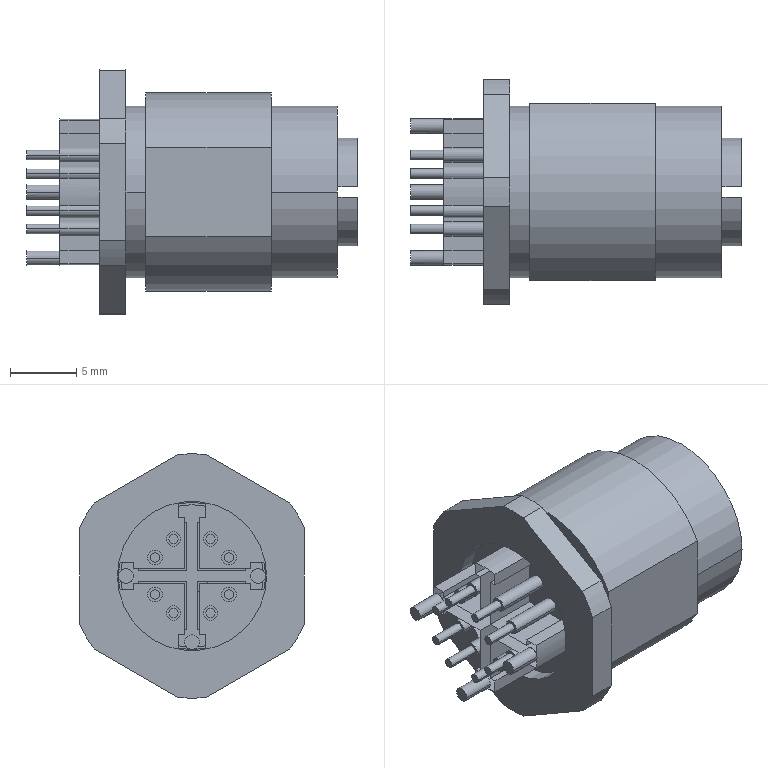Part | NX | features BREP 1 | 1 solid | 161 faces | box 25 x 17 x 18.5 mm | volume 2518 mm3 | plane 82 | cylinder 79 | commonest cylinder face diameters 0.7 x32 1.1 x22 18.5 x6 11.1 x5 8.2 x4 13 x4